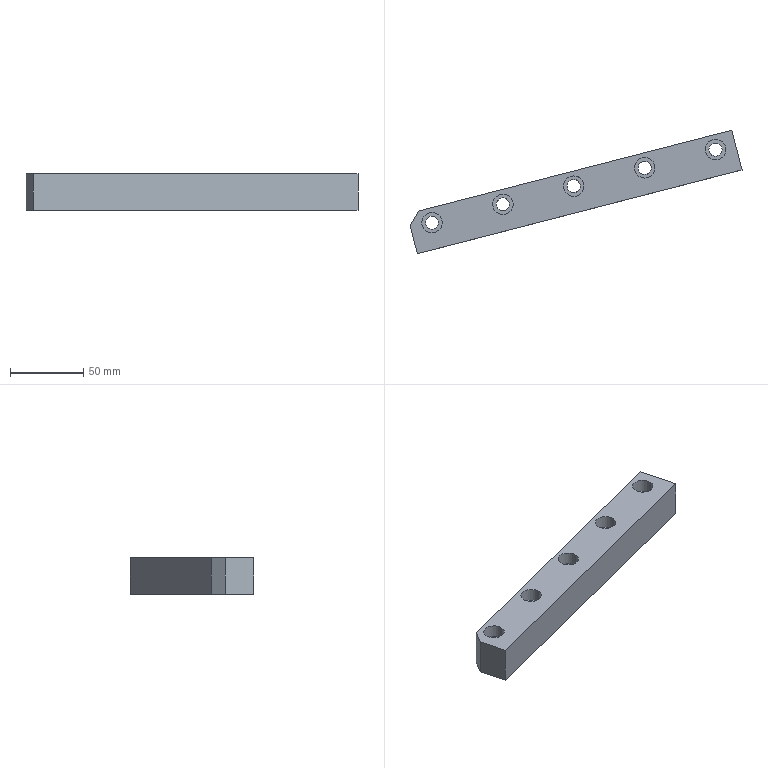Part | STEP file | 车灯-后视镜_id262_x_t | 1 solid | 22 faces | box 226.748 x 84.296 x 25 mm | volume 147489 mm3 | plane 12 | cylinder 10 | commonest cylinder face diameters 9 x5 14 x5
STEP:
#1=CARTESIAN_POINT('',(-453.609,15.169,-25.286));
#2=VERTEX_POINT('',#1);
#3=CARTESIAN_POINT('',(-454.732,19.526,-25.286));
#4=DIRECTION('',(0.,0.,1.));
#5=DIRECTION('',(0.2497,-0.9683,0.));
#6=AXIS2_PLACEMENT_3D('',#3,#4,#5);
#7=CIRCLE('',#6,4.5);
#8=EDGE_CURVE('',#2,#2,#7,.T.);
#9=ORIENTED_EDGE('',*,*,#8,.T.);
#10=EDGE_LOOP('',(#9));
#11=FACE_BOUND('',#10,.T.);
#12=CARTESIAN_POINT('',(-405.192,27.654,-25.286));
#13=VERTEX_POINT('',#12);
#14=CARTESIAN_POINT('',(-406.316,32.011,-25.286));
#15=DIRECTION('',(0.,0.,1.));
#16=DIRECTION('',(0.2497,-0.9683,0.));
#17=AXIS2_PLACEMENT_3D('',#14,#15,#16);
#18=CIRCLE('',#17,4.5);
#19=EDGE_CURVE('',#13,#13,#18,.T.);
#20=ORIENTED_EDGE('',*,*,#19,.T.);
#21=EDGE_LOOP('',(#20));
#22=FACE_BOUND('',#21,.T.);
#23=CARTESIAN_POINT('',(-356.776,40.139,-25.286));
#24=VERTEX_POINT('',#23);
#25=CARTESIAN_POINT('',(-357.9,44.496,-25.286));
#26=DIRECTION('',(0.,0.,1.));
#27=DIRECTION('',(0.2497,-0.9683,0.));
#28=AXIS2_PLACEMENT_3D('',#25,#26,#27);
#29=CIRCLE('',#28,4.5);
#30=EDGE_CURVE('',#24,#24,#29,.T.);
#31=ORIENTED_EDGE('',*,*,#30,.T.);
#32=EDGE_LOOP('',(#31));
#33=FACE_BOUND('',#32,.T.);
#34=CARTESIAN_POINT('',(-308.36,52.624,-25.286));
#35=VERTEX_POINT('',#34);
#36=CARTESIAN_POINT('',(-309.484,56.981,-25.286));
#37=DIRECTION('',(0.,0.,1.));
#38=DIRECTION('',(0.2497,-0.9683,0.));
#39=AXIS2_PLACEMENT_3D('',#36,#37,#38);
#40=CIRCLE('',#39,4.5);
#41=EDGE_CURVE('',#35,#35,#40,.T.);
#42=ORIENTED_EDGE('',*,*,#41,.T.);
#43=EDGE_LOOP('',(#42));
#44=FACE_BOUND('',#43,.T.);
#45=CARTESIAN_POINT('',(-259.944,65.109,-25.286));
#46=VERTEX_POINT('',#45);
#47=CARTESIAN_POINT('',(-261.068,69.466,-25.286));
#48=DIRECTION('',(0.,0.,1.));
#49=DIRECTION('',(0.2497,-0.9683,0.));
#50=AXIS2_PLACEMENT_3D('',#47,#48,#49);
#51=CIRCLE('',#50,4.5);
#52=EDGE_CURVE('',#46,#46,#51,.T.);
#53=ORIENTED_EDGE('',*,*,#52,.T.);
#54=EDGE_LOOP('',(#53));
#55=FACE_BOUND('',#54,.T.);
#56=CARTESIAN_POINT('',(-464.763,-1.649,-25.286));
#57=VERTEX_POINT('',#56);
#58=CARTESIAN_POINT('',(-469.757,17.717,-25.286));
#59=VERTEX_POINT('',#58);
#60=CARTESIAN_POINT('',(-464.763,-1.649,-25.286));
#61=DIRECTION('',(-0.2497,0.9683,0.));
#62=VECTOR('',#61,1.);
#63=LINE('',#60,#62);
#64=EDGE_CURVE('',#57,#59,#63,.T.);
#65=ORIENTED_EDGE('',*,*,#64,.T.);
#66=CARTESIAN_POINT('',(-464.008,27.462,-25.286));
#67=VERTEX_POINT('',#66);
#68=CARTESIAN_POINT('',(-464.008,27.462,-25.286));
#69=DIRECTION('',(0.5081,0.8613,0.));
#70=VECTOR('',#69,1.);
#71=LINE('',#68,#70);
#72=EDGE_CURVE('',#59,#67,#71,.T.);
#73=ORIENTED_EDGE('',*,*,#72,.T.);
#74=CARTESIAN_POINT('',(-250.,82.647,-25.286));
#75=VERTEX_POINT('',#74);
#76=CARTESIAN_POINT('',(-113.474,117.853,-25.286));
#77=DIRECTION('',(-0.9683,-0.2497,0.));
#78=VECTOR('',#77,1.);
#79=LINE('',#76,#78);
#80=EDGE_CURVE('',#75,#67,#79,.T.);
#81=ORIENTED_EDGE('',*,*,#80,.F.);
#82=CARTESIAN_POINT('',(-243.008,55.534,-25.286));
#83=VERTEX_POINT('',#82);
#84=CARTESIAN_POINT('',(-243.008,55.534,-25.286));
#85=DIRECTION('',(0.2497,-0.9683,0.));
#86=VECTOR('',#85,1.);
#87=LINE('',#84,#86);
#88=EDGE_CURVE('',#75,#83,#87,.T.);
#89=ORIENTED_EDGE('',*,*,#88,.T.);
#90=CARTESIAN_POINT('',(-106.483,90.74,-25.286));
#91=DIRECTION('',(-0.9683,-0.2497,0.));
#92=VECTOR('',#91,1.);
#93=LINE('',#90,#92);
#94=EDGE_CURVE('',#83,#57,#93,.T.);
#95=ORIENTED_EDGE('',*,*,#94,.T.);
#96=EDGE_LOOP('',(#65,#73,#81,#89,#95));
#97=FACE_BOUND('',#96,.T.);
#98=CARTESIAN_POINT('',(-106.483,90.74,-25.286));
#99=DIRECTION('',(0.,0.,-1.));
#100=DIRECTION('',(-0.9683,-0.2497,0.));
#101=AXIS2_PLACEMENT_3D('',#98,#99,#100);
#102=PLANE('',#101);
#103=ADVANCED_FACE('',(#11,#22,#33,#44,#55,#97),#102,.T.);
#104=CARTESIAN_POINT('',(-464.763,-1.649,-0.2856));
#105=VERTEX_POINT('',#104);
#106=CARTESIAN_POINT('',(-469.757,17.717,-0.2856));
#107=VERTEX_POINT('',#106);
#108=CARTESIAN_POINT('',(-483.305,70.259,-0.2856));
#109=DIRECTION('',(-0.2497,0.9683,0.));
#110=VECTOR('',#109,1.);
#111=LINE('',#108,#110);
#112=EDGE_CURVE('',#105,#107,#111,.T.);
#113=ORIENTED_EDGE('',*,*,#112,.T.);
#114=CARTESIAN_POINT('',(-469.757,17.717,-100.5));
#115=DIRECTION('',(0.,0.,-1.));
#116=VECTOR('',#115,1.);
#117=LINE('',#114,#116);
#118=EDGE_CURVE('',#107,#59,#117,.T.);
#119=ORIENTED_EDGE('',*,*,#118,.T.);
#120=ORIENTED_EDGE('',*,*,#64,.F.);
#121=CARTESIAN_POINT('',(-464.763,-1.649,-25.286));
#122=DIRECTION('',(0.,0.,1.));
#123=VECTOR('',#122,1.);
#124=LINE('',#121,#123);
#125=EDGE_CURVE('',#57,#105,#124,.T.);
#126=ORIENTED_EDGE('',*,*,#125,.T.);
#127=EDGE_LOOP('',(#113,#119,#120,#126));
#128=FACE_OUTER_BOUND('',#127,.T.);
#129=CARTESIAN_POINT('',(-483.305,70.259,-100.5));
#130=DIRECTION('',(-0.9683,-0.2497,0.));
#131=DIRECTION('',(0.2497,-0.9683,0.));
#132=AXIS2_PLACEMENT_3D('',#129,#130,#131);
#133=PLANE('',#132);
#134=ADVANCED_FACE('',(#128),#133,.T.);
#135=CARTESIAN_POINT('',(-452.984,12.748,-0.2856));
#136=VERTEX_POINT('',#135);
#137=CARTESIAN_POINT('',(-454.732,19.526,-0.2856));
#138=DIRECTION('',(0.,0.,-1.));
#139=DIRECTION('',(0.2497,-0.9683,0.));
#140=AXIS2_PLACEMENT_3D('',#137,#138,#139);
#141=CIRCLE('',#140,7.);
#142=EDGE_CURVE('',#136,#136,#141,.T.);
#143=ORIENTED_EDGE('',*,*,#142,.T.);
#144=EDGE_LOOP('',(#143));
#145=FACE_BOUND('',#144,.T.);
#146=CARTESIAN_POINT('',(-404.568,25.233,-0.2856));
#147=VERTEX_POINT('',#146);
#148=CARTESIAN_POINT('',(-406.316,32.011,-0.2856));
#149=DIRECTION('',(0.,0.,-1.));
#150=DIRECTION('',(0.2497,-0.9683,0.));
#151=AXIS2_PLACEMENT_3D('',#148,#149,#150);
#152=CIRCLE('',#151,7.);
#153=EDGE_CURVE('',#147,#147,#152,.T.);
#154=ORIENTED_EDGE('',*,*,#153,.T.);
#155=EDGE_LOOP('',(#154));
#156=FACE_BOUND('',#155,.T.);
#157=CARTESIAN_POINT('',(-356.152,37.718,-0.2856));
#158=VERTEX_POINT('',#157);
#159=CARTESIAN_POINT('',(-357.9,44.496,-0.2856));
#160=DIRECTION('',(0.,0.,-1.));
#161=DIRECTION('',(0.2497,-0.9683,0.));
#162=AXIS2_PLACEMENT_3D('',#159,#160,#161);
#163=CIRCLE('',#162,7.);
#164=EDGE_CURVE('',#158,#158,#163,.T.);
#165=ORIENTED_EDGE('',*,*,#164,.T.);
#166=EDGE_LOOP('',(#165));
#167=FACE_BOUND('',#166,.T.);
#168=CARTESIAN_POINT('',(-307.736,50.203,-0.2856));
#169=VERTEX_POINT('',#168);
#170=CARTESIAN_POINT('',(-309.484,56.981,-0.2856));
#171=DIRECTION('',(0.,0.,-1.));
#172=DIRECTION('',(0.2497,-0.9683,0.));
#173=AXIS2_PLACEMENT_3D('',#170,#171,#172);
#174=CIRCLE('',#173,7.);
#175=EDGE_CURVE('',#169,#169,#174,.T.);
#176=ORIENTED_EDGE('',*,*,#175,.T.);
#177=EDGE_LOOP('',(#176));
#178=FACE_BOUND('',#177,.T.);
#179=CARTESIAN_POINT('',(-259.32,62.688,-0.2856));
#180=VERTEX_POINT('',#179);
#181=CARTESIAN_POINT('',(-261.068,69.466,-0.2856));
#182=DIRECTION('',(0.,0.,-1.));
#183=DIRECTION('',(0.2497,-0.9683,0.));
#184=AXIS2_PLACEMENT_3D('',#181,#182,#183);
#185=CIRCLE('',#184,7.);
#186=EDGE_CURVE('',#180,#180,#185,.T.);
#187=ORIENTED_EDGE('',*,*,#186,.T.);
#188=EDGE_LOOP('',(#187));
#189=FACE_BOUND('',#188,.T.);
#190=CARTESIAN_POINT('',(-250.,82.647,-0.2856));
#191=VERTEX_POINT('',#190);
#192=CARTESIAN_POINT('',(-464.008,27.462,-0.2856));
#193=VERTEX_POINT('',#192);
#194=CARTESIAN_POINT('',(-113.474,117.853,-0.2856));
#195=DIRECTION('',(-0.9683,-0.2497,0.));
#196=VECTOR('',#195,1.);
#197=LINE('',#194,#196);
#198=EDGE_CURVE('',#191,#193,#197,.T.);
#199=ORIENTED_EDGE('',*,*,#198,.T.);
#200=CARTESIAN_POINT('',(-464.008,27.462,-0.2856));
#201=DIRECTION('',(-0.5081,-0.8613,0.));
#202=VECTOR('',#201,1.);
#203=LINE('',#200,#202);
#204=EDGE_CURVE('',#193,#107,#203,.T.);
#205=ORIENTED_EDGE('',*,*,#204,.T.);
#206=ORIENTED_EDGE('',*,*,#112,.F.);
#207=CARTESIAN_POINT('',(-243.008,55.534,-0.2856));
#208=VERTEX_POINT('',#207);
#209=CARTESIAN_POINT('',(-106.483,90.74,-0.2856));
#210=DIRECTION('',(-0.9683,-0.2497,0.));
#211=VECTOR('',#210,1.);
#212=LINE('',#209,#211);
#213=EDGE_CURVE('',#208,#105,#212,.T.);
#214=ORIENTED_EDGE('',*,*,#213,.F.);
#215=CARTESIAN_POINT('',(-243.008,55.534,-0.2856));
#216=DIRECTION('',(-0.2497,0.9683,0.));
#217=VECTOR('',#216,1.);
#218=LINE('',#215,#217);
#219=EDGE_CURVE('',#208,#191,#218,.T.);
#220=ORIENTED_EDGE('',*,*,#219,.T.);
#221=EDGE_LOOP('',(#199,#205,#206,#214,#220));
#222=FACE_BOUND('',#221,.T.);
#223=CARTESIAN_POINT('',(-106.483,90.74,-0.2856));
#224=DIRECTION('',(0.,0.,-1.));
#225=DIRECTION('',(-0.9683,-0.2497,0.));
#226=AXIS2_PLACEMENT_3D('',#223,#224,#225);
#227=PLANE('',#226);
#228=ADVANCED_FACE('',(#145,#156,#167,#178,#189,#222),#227,.F.);
#229=ORIENTED_EDGE('',*,*,#80,.T.);
#230=CARTESIAN_POINT('',(-464.008,27.462,-25.286));
#231=DIRECTION('',(0.,0.,1.));
#232=VECTOR('',#231,1.);
#233=LINE('',#230,#232);
#234=EDGE_CURVE('',#67,#193,#233,.T.);
#235=ORIENTED_EDGE('',*,*,#234,.T.);
#236=ORIENTED_EDGE('',*,*,#198,.F.);
#237=CARTESIAN_POINT('',(-250.,82.647,-25.286));
#238=DIRECTION('',(0.,0.,-1.));
#239=VECTOR('',#238,1.);
#240=LINE('',#237,#239);
#241=EDGE_CURVE('',#191,#75,#240,.T.);
#242=ORIENTED_EDGE('',*,*,#241,.T.);
#243=EDGE_LOOP('',(#229,#235,#236,#242));
#244=FACE_OUTER_BOUND('',#243,.T.);
#245=CARTESIAN_POINT('',(-113.474,117.853,-25.286));
#246=DIRECTION('',(0.2497,-0.9683,0.));
#247=DIRECTION('',(-0.9683,-0.2497,0.));
#248=AXIS2_PLACEMENT_3D('',#245,#246,#247);
#249=PLANE('',#248);
#250=ADVANCED_FACE('',(#244),#249,.F.);
#251=CARTESIAN_POINT('',(-243.008,55.534,-25.286));
#252=DIRECTION('',(0.,0.,-1.));
#253=VECTOR('',#252,1.);
#254=LINE('',#251,#253);
#255=EDGE_CURVE('',#208,#83,#254,.T.);
#256=ORIENTED_EDGE('',*,*,#255,.F.);
#257=ORIENTED_EDGE('',*,*,#213,.T.);
#258=ORIENTED_EDGE('',*,*,#125,.F.);
#259=ORIENTED_EDGE('',*,*,#94,.F.);
#260=EDGE_LOOP('',(#256,#257,#258,#259));
#261=FACE_OUTER_BOUND('',#260,.T.);
#262=CARTESIAN_POINT('',(-106.483,90.74,-25.286));
#263=DIRECTION('',(0.2497,-0.9683,0.));
#264=DIRECTION('',(-0.9683,-0.2497,0.));
#265=AXIS2_PLACEMENT_3D('',#262,#263,#264);
#266=PLANE('',#265);
#267=ADVANCED_FACE('',(#261),#266,.T.);
#268=ORIENTED_EDGE('',*,*,#219,.F.);
#269=ORIENTED_EDGE('',*,*,#255,.T.);
#270=ORIENTED_EDGE('',*,*,#88,.F.);
#271=ORIENTED_EDGE('',*,*,#241,.F.);
#272=EDGE_LOOP('',(#268,#269,#270,#271));
#273=FACE_OUTER_BOUND('',#272,.T.);
#274=CARTESIAN_POINT('',(-250.,82.647,-0.5));
#275=DIRECTION('',(-0.9683,-0.2497,0.));
#276=DIRECTION('',(0.2497,-0.9683,0.));
#277=AXIS2_PLACEMENT_3D('',#274,#275,#276);
#278=PLANE('',#277);
#279=ADVANCED_FACE('',(#273),#278,.F.);
#280=CARTESIAN_POINT('',(-265.568,69.466,-9.286));
#281=VERTEX_POINT('',#280);
#282=CARTESIAN_POINT('',(-261.068,69.466,-9.286));
#283=DIRECTION('',(0.,0.,1.));
#284=DIRECTION('',(-1.,0.,0.));
#285=AXIS2_PLACEMENT_3D('',#282,#283,#284);
#286=CIRCLE('',#285,4.5);
#287=EDGE_CURVE('',#281,#281,#286,.T.);
#288=ORIENTED_EDGE('',*,*,#287,.T.);
#289=EDGE_LOOP('',(#288));
#290=FACE_BOUND('',#289,.T.);
#291=ORIENTED_EDGE('',*,*,#52,.F.);
#292=EDGE_LOOP('',(#291));
#293=FACE_BOUND('',#292,.T.);
#294=CARTESIAN_POINT('',(-261.068,69.466,-24.786));
#295=DIRECTION('',(0.,0.,1.));
#296=DIRECTION('',(-0.2497,0.9683,0.));
#297=AXIS2_PLACEMENT_3D('',#294,#295,#296);
#298=CYLINDRICAL_SURFACE('',#297,4.5);
#299=ADVANCED_FACE('',(#290,#293),#298,.F.);
#300=ORIENTED_EDGE('',*,*,#287,.F.);
#301=EDGE_LOOP('',(#300));
#302=FACE_BOUND('',#301,.T.);
#303=CARTESIAN_POINT('',(-262.815,76.244,-9.286));
#304=VERTEX_POINT('',#303);
#305=CARTESIAN_POINT('',(-261.068,69.466,-9.286));
#306=DIRECTION('',(0.,0.,1.));
#307=DIRECTION('',(-0.2497,0.9683,0.));
#308=AXIS2_PLACEMENT_3D('',#305,#306,#307);
#309=CIRCLE('',#308,7.);
#310=EDGE_CURVE('',#304,#304,#309,.T.);
#311=ORIENTED_EDGE('',*,*,#310,.T.);
#312=EDGE_LOOP('',(#311));
#313=FACE_BOUND('',#312,.T.);
#314=CARTESIAN_POINT('',(-261.068,69.466,-9.286));
#315=DIRECTION('',(0.,0.,-1.));
#316=DIRECTION('',(0.2497,-0.9683,0.));
#317=AXIS2_PLACEMENT_3D('',#314,#315,#316);
#318=PLANE('',#317);
#319=ADVANCED_FACE('',(#302,#313),#318,.F.);
#320=ORIENTED_EDGE('',*,*,#310,.F.);
#321=EDGE_LOOP('',(#320));
#322=FACE_BOUND('',#321,.T.);
#323=ORIENTED_EDGE('',*,*,#186,.F.);
#324=EDGE_LOOP('',(#323));
#325=FACE_BOUND('',#324,.T.);
#326=CARTESIAN_POINT('',(-261.068,69.466,-0.2856));
#327=DIRECTION('',(0.,0.,-1.));
#328=DIRECTION('',(0.2497,-0.9683,0.));
#329=AXIS2_PLACEMENT_3D('',#326,#327,#328);
#330=CYLINDRICAL_SURFACE('',#329,7.);
#331=ADVANCED_FACE('',(#322,#325),#330,.F.);
#332=CARTESIAN_POINT('',(-313.984,56.981,-9.286));
#333=VERTEX_POINT('',#332);
#334=CARTESIAN_POINT('',(-309.484,56.981,-9.286));
#335=DIRECTION('',(0.,0.,1.));
#336=DIRECTION('',(-1.,0.,0.));
#337=AXIS2_PLACEMENT_3D('',#334,#335,#336);
#338=CIRCLE('',#337,4.5);
#339=EDGE_CURVE('',#333,#333,#338,.T.);
#340=ORIENTED_EDGE('',*,*,#339,.T.);
#341=EDGE_LOOP('',(#340));
#342=FACE_BOUND('',#341,.T.);
#343=ORIENTED_EDGE('',*,*,#41,.F.);
#344=EDGE_LOOP('',(#343));
#345=FACE_BOUND('',#344,.T.);
#346=CARTESIAN_POINT('',(-309.484,56.981,-24.786));
#347=DIRECTION('',(0.,0.,1.));
#348=DIRECTION('',(-0.2497,0.9683,0.));
#349=AXIS2_PLACEMENT_3D('',#346,#347,#348);
#350=CYLINDRICAL_SURFACE('',#349,4.5);
#351=ADVANCED_FACE('',(#342,#345),#350,.F.);
#352=ORIENTED_EDGE('',*,*,#339,.F.);
#353=EDGE_LOOP('',(#352));
#354=FACE_BOUND('',#353,.T.);
#355=CARTESIAN_POINT('',(-311.232,63.759,-9.286));
#356=VERTEX_POINT('',#355);
#357=CARTESIAN_POINT('',(-309.484,56.981,-9.286));
#358=DIRECTION('',(0.,0.,1.));
#359=DIRECTION('',(-0.2497,0.9683,0.));
#360=AXIS2_PLACEMENT_3D('',#357,#358,#359);
#361=CIRCLE('',#360,7.);
#362=EDGE_CURVE('',#356,#356,#361,.T.);
#363=ORIENTED_EDGE('',*,*,#362,.T.);
#364=EDGE_LOOP('',(#363));
#365=FACE_BOUND('',#364,.T.);
#366=CARTESIAN_POINT('',(-309.484,56.981,-9.286));
#367=DIRECTION('',(0.,0.,-1.));
#368=DIRECTION('',(0.2497,-0.9683,0.));
#369=AXIS2_PLACEMENT_3D('',#366,#367,#368);
#370=PLANE('',#369);
#371=ADVANCED_FACE('',(#354,#365),#370,.F.);
#372=ORIENTED_EDGE('',*,*,#362,.F.);
#373=EDGE_LOOP('',(#372));
#374=FACE_BOUND('',#373,.T.);
#375=ORIENTED_EDGE('',*,*,#175,.F.);
#376=EDGE_LOOP('',(#375));
#377=FACE_BOUND('',#376,.T.);
#378=CARTESIAN_POINT('',(-309.484,56.981,-0.2856));
#379=DIRECTION('',(0.,0.,-1.));
#380=DIRECTION('',(0.2497,-0.9683,0.));
#381=AXIS2_PLACEMENT_3D('',#378,#379,#380);
#382=CYLINDRICAL_SURFACE('',#381,7.);
#383=ADVANCED_FACE('',(#374,#377),#382,.F.);
#384=CARTESIAN_POINT('',(-362.4,44.496,-9.286));
#385=VERTEX_POINT('',#384);
#386=CARTESIAN_POINT('',(-357.9,44.496,-9.286));
#387=DIRECTION('',(0.,0.,1.));
#388=DIRECTION('',(-1.,0.,0.));
#389=AXIS2_PLACEMENT_3D('',#386,#387,#388);
#390=CIRCLE('',#389,4.5);
#391=EDGE_CURVE('',#385,#385,#390,.T.);
#392=ORIENTED_EDGE('',*,*,#391,.T.);
#393=EDGE_LOOP('',(#392));
#394=FACE_BOUND('',#393,.T.);
#395=ORIENTED_EDGE('',*,*,#30,.F.);
#396=EDGE_LOOP('',(#395));
#397=FACE_BOUND('',#396,.T.);
#398=CARTESIAN_POINT('',(-357.9,44.496,-24.786));
#399=DIRECTION('',(0.,0.,1.));
#400=DIRECTION('',(-0.2497,0.9683,0.));
#401=AXIS2_PLACEMENT_3D('',#398,#399,#400);
#402=CYLINDRICAL_SURFACE('',#401,4.5);
#403=ADVANCED_FACE('',(#394,#397),#402,.F.);
#404=ORIENTED_EDGE('',*,*,#391,.F.);
#405=EDGE_LOOP('',(#404));
#406=FACE_BOUND('',#405,.T.);
#407=CARTESIAN_POINT('',(-359.648,51.274,-9.286));
#408=VERTEX_POINT('',#407);
#409=CARTESIAN_POINT('',(-357.9,44.496,-9.286));
#410=DIRECTION('',(0.,0.,1.));
#411=DIRECTION('',(-0.2497,0.9683,0.));
#412=AXIS2_PLACEMENT_3D('',#409,#410,#411);
#413=CIRCLE('',#412,7.);
#414=EDGE_CURVE('',#408,#408,#413,.T.);
#415=ORIENTED_EDGE('',*,*,#414,.T.);
#416=EDGE_LOOP('',(#415));
#417=FACE_BOUND('',#416,.T.);
#418=CARTESIAN_POINT('',(-357.9,44.496,-9.286));
#419=DIRECTION('',(0.,0.,-1.));
#420=DIRECTION('',(0.2497,-0.9683,0.));
#421=AXIS2_PLACEMENT_3D('',#418,#419,#420);
#422=PLANE('',#421);
#423=ADVANCED_FACE('',(#406,#417),#422,.F.);
#424=ORIENTED_EDGE('',*,*,#414,.F.);
#425=EDGE_LOOP('',(#424));
#426=FACE_BOUND('',#425,.T.);
#427=ORIENTED_EDGE('',*,*,#164,.F.);
#428=EDGE_LOOP('',(#427));
#429=FACE_BOUND('',#428,.T.);
#430=CARTESIAN_POINT('',(-357.9,44.496,-0.2856));
#431=DIRECTION('',(0.,0.,-1.));
#432=DIRECTION('',(0.2497,-0.9683,0.));
#433=AXIS2_PLACEMENT_3D('',#430,#431,#432);
#434=CYLINDRICAL_SURFACE('',#433,7.);
#435=ADVANCED_FACE('',(#426,#429),#434,.F.);
#436=CARTESIAN_POINT('',(-410.816,32.011,-9.286));
#437=VERTEX_POINT('',#436);
#438=CARTESIAN_POINT('',(-406.316,32.011,-9.286));
#439=DIRECTION('',(0.,0.,1.));
#440=DIRECTION('',(-1.,0.,0.));
#441=AXIS2_PLACEMENT_3D('',#438,#439,#440);
#442=CIRCLE('',#441,4.5);
#443=EDGE_CURVE('',#437,#437,#442,.T.);
#444=ORIENTED_EDGE('',*,*,#443,.T.);
#445=EDGE_LOOP('',(#444));
#446=FACE_BOUND('',#445,.T.);
#447=ORIENTED_EDGE('',*,*,#19,.F.);
#448=EDGE_LOOP('',(#447));
#449=FACE_BOUND('',#448,.T.);
#450=CARTESIAN_POINT('',(-406.316,32.011,-24.786));
#451=DIRECTION('',(0.,0.,1.));
#452=DIRECTION('',(-0.2497,0.9683,0.));
#453=AXIS2_PLACEMENT_3D('',#450,#451,#452);
#454=CYLINDRICAL_SURFACE('',#453,4.5);
#455=ADVANCED_FACE('',(#446,#449),#454,.F.);
#456=ORIENTED_EDGE('',*,*,#443,.F.);
#457=EDGE_LOOP('',(#456));
#458=FACE_BOUND('',#457,.T.);
#459=CARTESIAN_POINT('',(-408.064,38.79,-9.286));
#460=VERTEX_POINT('',#459);
#461=CARTESIAN_POINT('',(-406.316,32.011,-9.286));
#462=DIRECTION('',(0.,0.,1.));
#463=DIRECTION('',(-0.2497,0.9683,0.));
#464=AXIS2_PLACEMENT_3D('',#461,#462,#463);
#465=CIRCLE('',#464,7.);
#466=EDGE_CURVE('',#460,#460,#465,.T.);
#467=ORIENTED_EDGE('',*,*,#466,.T.);
#468=EDGE_LOOP('',(#467));
#469=FACE_BOUND('',#468,.T.);
#470=CARTESIAN_POINT('',(-406.316,32.011,-9.286));
#471=DIRECTION('',(0.,0.,-1.));
#472=DIRECTION('',(0.2497,-0.9683,0.));
#473=AXIS2_PLACEMENT_3D('',#470,#471,#472);
#474=PLANE('',#473);
#475=ADVANCED_FACE('',(#458,#469),#474,.F.);
#476=ORIENTED_EDGE('',*,*,#466,.F.);
#477=EDGE_LOOP('',(#476));
#478=FACE_BOUND('',#477,.T.);
#479=ORIENTED_EDGE('',*,*,#153,.F.);
#480=EDGE_LOOP('',(#479));
#481=FACE_BOUND('',#480,.T.);
#482=CARTESIAN_POINT('',(-406.316,32.011,-0.2856));
#483=DIRECTION('',(0.,0.,-1.));
#484=DIRECTION('',(0.2497,-0.9683,0.));
#485=AXIS2_PLACEMENT_3D('',#482,#483,#484);
#486=CYLINDRICAL_SURFACE('',#485,7.);
#487=ADVANCED_FACE('',(#478,#481),#486,.F.);
#488=CARTESIAN_POINT('',(-459.232,19.526,-9.286));
#489=VERTEX_POINT('',#488);
#490=CARTESIAN_POINT('',(-454.732,19.526,-9.286));
#491=DIRECTION('',(0.,0.,1.));
#492=DIRECTION('',(-1.,0.,0.));
#493=AXIS2_PLACEMENT_3D('',#490,#491,#492);
#494=CIRCLE('',#493,4.5);
#495=EDGE_CURVE('',#489,#489,#494,.T.);
#496=ORIENTED_EDGE('',*,*,#495,.T.);
#497=EDGE_LOOP('',(#496));
#498=FACE_BOUND('',#497,.T.);
#499=ORIENTED_EDGE('',*,*,#8,.F.);
#500=EDGE_LOOP('',(#499));
#501=FACE_BOUND('',#500,.T.);
#502=CARTESIAN_POINT('',(-454.732,19.526,-24.786));
#503=DIRECTION('',(0.,0.,1.));
#504=DIRECTION('',(-0.2497,0.9683,0.));
#505=AXIS2_PLACEMENT_3D('',#502,#503,#504);
#506=CYLINDRICAL_SURFACE('',#505,4.5);
#507=ADVANCED_FACE('',(#498,#501),#506,.F.);
#508=ORIENTED_EDGE('',*,*,#495,.F.);
#509=EDGE_LOOP('',(#508));
#510=FACE_BOUND('',#509,.T.);
#511=CARTESIAN_POINT('',(-456.48,26.305,-9.286));
#512=VERTEX_POINT('',#511);
#513=CARTESIAN_POINT('',(-454.732,19.526,-9.286));
#514=DIRECTION('',(0.,0.,1.));
#515=DIRECTION('',(-0.2497,0.9683,0.));
#516=AXIS2_PLACEMENT_3D('',#513,#514,#515);
#517=CIRCLE('',#516,7.);
#518=EDGE_CURVE('',#512,#512,#517,.T.);
#519=ORIENTED_EDGE('',*,*,#518,.T.);
#520=EDGE_LOOP('',(#519));
#521=FACE_BOUND('',#520,.T.);
#522=CARTESIAN_POINT('',(-454.732,19.526,-9.286));
#523=DIRECTION('',(0.,0.,-1.));
#524=DIRECTION('',(0.2497,-0.9683,0.));
#525=AXIS2_PLACEMENT_3D('',#522,#523,#524);
#526=PLANE('',#525);
#527=ADVANCED_FACE('',(#510,#521),#526,.F.);
#528=ORIENTED_EDGE('',*,*,#518,.F.);
#529=EDGE_LOOP('',(#528));
#530=FACE_BOUND('',#529,.T.);
#531=ORIENTED_EDGE('',*,*,#142,.F.);
#532=EDGE_LOOP('',(#531));
#533=FACE_BOUND('',#532,.T.);
#534=CARTESIAN_POINT('',(-454.732,19.526,-0.2856));
#535=DIRECTION('',(0.,0.,-1.));
#536=DIRECTION('',(0.2497,-0.9683,0.));
#537=AXIS2_PLACEMENT_3D('',#534,#535,#536);
#538=CYLINDRICAL_SURFACE('',#537,7.);
#539=ADVANCED_FACE('',(#530,#533),#538,.F.);
#540=ORIENTED_EDGE('',*,*,#72,.F.);
#541=ORIENTED_EDGE('',*,*,#118,.F.);
#542=ORIENTED_EDGE('',*,*,#204,.F.);
#543=ORIENTED_EDGE('',*,*,#234,.F.);
#544=EDGE_LOOP('',(#540,#541,#542,#543));
#545=FACE_OUTER_BOUND('',#544,.T.);
#546=CARTESIAN_POINT('',(-464.008,27.462,-25.286));
#547=DIRECTION('',(-0.8613,0.5081,0.));
#548=DIRECTION('',(-0.5081,-0.8613,0.));
#549=AXIS2_PLACEMENT_3D('',#546,#547,#548);
#550=PLANE('',#549);
#551=ADVANCED_FACE('',(#545),#550,.T.);
#552=CLOSED_SHELL('',(#103,#134,#228,#250,#267,#279,#299,#319,#331,#351,#371,#383,#403,#423,#435,#455,#475,#487,#507,#527,#539,#551));
#553=MANIFOLD_SOLID_BREP('',#552);
#554=(LENGTH_UNIT()NAMED_UNIT(*)SI_UNIT(.MILLI.,.METRE.));
#555=UNCERTAINTY_MEASURE_WITH_UNIT(LENGTH_MEASURE(0.00002),#554,'','');
#556=(NAMED_UNIT(*)PLANE_ANGLE_UNIT()SI_UNIT($,.RADIAN.));
#557=PLANE_ANGLE_MEASURE_WITH_UNIT(PLANE_ANGLE_MEASURE(0.01745),#556);
#558=DIMENSIONAL_EXPONENTS(0.,0.,0.,0.,0.,0.,0.);
#559=(CONVERSION_BASED_UNIT('DEGREE',#557)NAMED_UNIT(#558)PLANE_ANGLE_UNIT());
#560=(NAMED_UNIT(*)SI_UNIT($,.STERADIAN.)SOLID_ANGLE_UNIT());
#561=(GEOMETRIC_REPRESENTATION_CONTEXT(3)GLOBAL_UNCERTAINTY_ASSIGNED_CONTEXT((#555))GLOBAL_UNIT_ASSIGNED_CONTEXT((#554,#559,#560))REPRESENTATION_CONTEXT('',''));
#562=ADVANCED_BREP_SHAPE_REPRESENTATION('',(#553),#561);